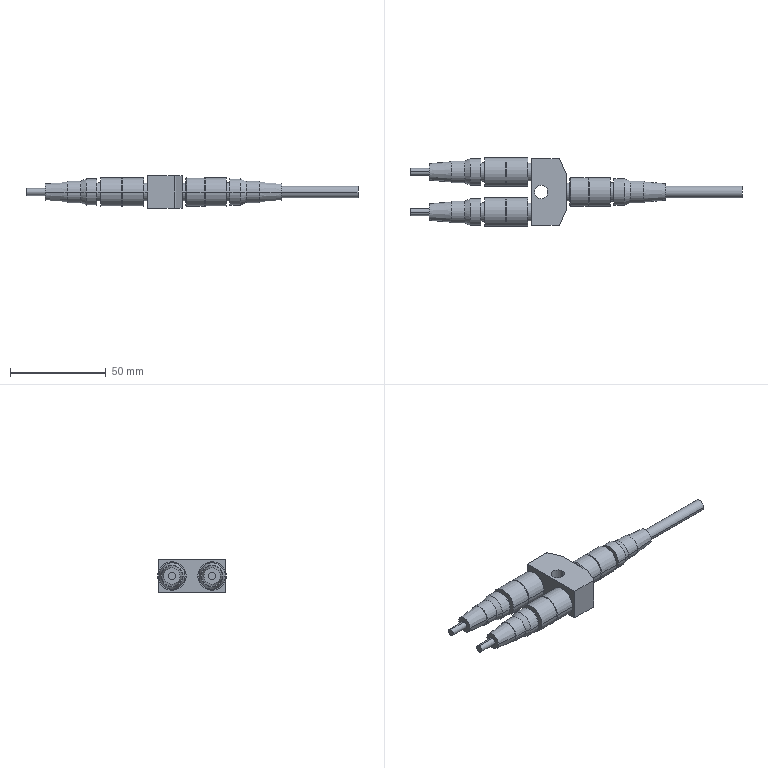Part | STEP file | [Y joint]-3 | 1 solid | 101 faces | box 173.6 x 35.9 x 17 mm | volume 31443 mm3 | cylinder 50 | plane 31 | cone 16 | torus 4 | commonest cylinder face diameters 14.9 x12 9.3 x6 9.6 x6 11.4 x6 13.8 x6 3.7 x4